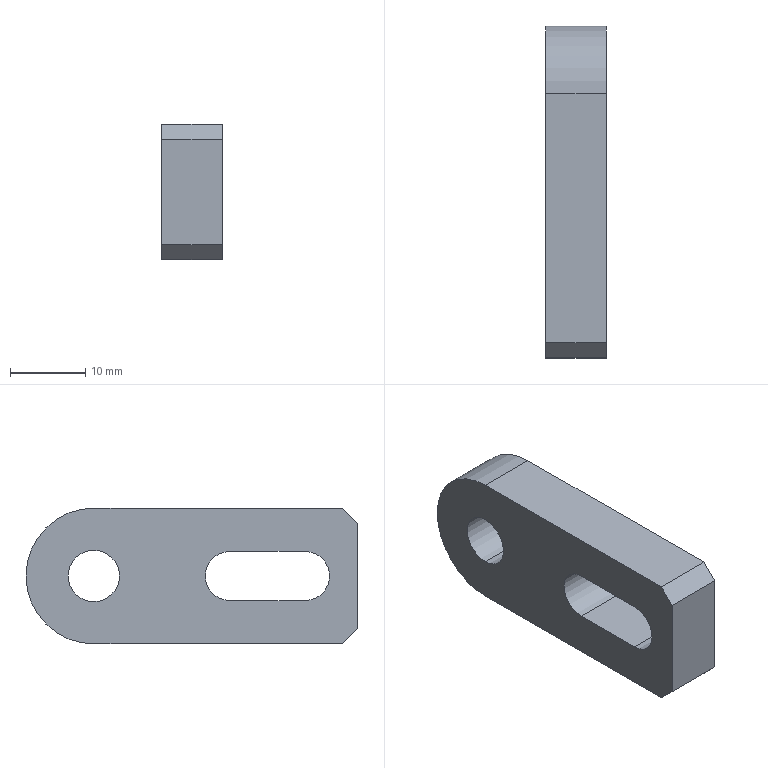Part | SolidWorks | features Chamfer 1, Extrusion 1, HoleWzd 1 | 1 solid | 14 faces | box 8 x 44 x 18 mm | volume 4950 mm3 | plane 9 | cylinder 5 | commonest cylinder face diameters 6.5 x2 6.8 x2 18 x1
STEP:
#1=CARTESIAN_POINT('',(4.,35.,3.4));
#2=VERTEX_POINT('',#1);
#3=CARTESIAN_POINT('',(4.,35.,-3.4));
#4=VERTEX_POINT('',#3);
#5=CARTESIAN_POINT('',(4.,35.,0.));
#6=DIRECTION('',(1.,0.,0.));
#7=DIRECTION('',(0.,0.,-1.));
#8=AXIS2_PLACEMENT_3D('',#5,#6,#7);
#9=CIRCLE('',#8,3.4);
#10=EDGE_CURVE('',#2,#4,#9,.T.);
#11=ORIENTED_EDGE('',*,*,#10,.T.);
#12=CARTESIAN_POINT('',(-4.,35.,-3.4));
#13=VERTEX_POINT('',#12);
#14=CARTESIAN_POINT('',(-4.,35.,-3.4));
#15=DIRECTION('',(-1.,0.,0.));
#16=VECTOR('',#15,1000.);
#17=LINE('',#14,#16);
#18=EDGE_CURVE('',#4,#13,#17,.T.);
#19=ORIENTED_EDGE('',*,*,#18,.T.);
#20=CARTESIAN_POINT('',(-4.,35.,3.4));
#21=VERTEX_POINT('',#20);
#22=CARTESIAN_POINT('',(-4.,35.,0.));
#23=DIRECTION('',(-1.,0.,0.));
#24=DIRECTION('',(0.,0.,1.));
#25=AXIS2_PLACEMENT_3D('',#22,#23,#24);
#26=CIRCLE('',#25,3.4);
#27=EDGE_CURVE('',#13,#21,#26,.T.);
#28=ORIENTED_EDGE('',*,*,#27,.T.);
#29=CARTESIAN_POINT('',(-4.,35.,3.4));
#30=DIRECTION('',(-1.,0.,0.));
#31=VECTOR('',#30,1000.);
#32=LINE('',#29,#31);
#33=EDGE_CURVE('',#2,#21,#32,.T.);
#34=ORIENTED_EDGE('',*,*,#33,.F.);
#35=EDGE_LOOP('',(#11,#19,#28,#34));
#36=FACE_OUTER_BOUND('',#35,.T.);
#37=CARTESIAN_POINT('',(-4.,35.,0.));
#38=DIRECTION('',(-1.,0.,0.));
#39=DIRECTION('',(0.,0.,1.));
#40=AXIS2_PLACEMENT_3D('',#37,#38,#39);
#41=CYLINDRICAL_SURFACE('',#40,3.4);
#42=ADVANCED_FACE('',(#36),#41,.F.);
#43=ORIENTED_EDGE('',*,*,#10,.F.);
#44=CARTESIAN_POINT('',(4.,35.,0.));
#45=DIRECTION('',(1.,0.,0.));
#46=DIRECTION('',(0.,0.,-1.));
#47=AXIS2_PLACEMENT_3D('',#44,#45,#46);
#48=CIRCLE('',#47,3.4);
#49=EDGE_CURVE('',#4,#2,#48,.T.);
#50=ORIENTED_EDGE('',*,*,#49,.F.);
#51=EDGE_LOOP('',(#43,#50));
#52=FACE_BOUND('',#51,.T.);
#53=CARTESIAN_POINT('',(4.,35.,9.));
#54=VERTEX_POINT('',#53);
#55=CARTESIAN_POINT('',(4.,2.,9.));
#56=VERTEX_POINT('',#55);
#57=CARTESIAN_POINT('',(4.,0.,9.));
#58=DIRECTION('',(0.,-1.,0.));
#59=VECTOR('',#58,1000.);
#60=LINE('',#57,#59);
#61=EDGE_CURVE('',#54,#56,#60,.T.);
#62=ORIENTED_EDGE('',*,*,#61,.T.);
#63=CARTESIAN_POINT('',(4.,0.,7.));
#64=VERTEX_POINT('',#63);
#65=CARTESIAN_POINT('',(4.,14.,21.));
#66=DIRECTION('',(0.,-0.7071,-0.7071));
#67=VECTOR('',#66,1000.);
#68=LINE('',#65,#67);
#69=EDGE_CURVE('',#56,#64,#68,.T.);
#70=ORIENTED_EDGE('',*,*,#69,.T.);
#71=CARTESIAN_POINT('',(4.,0.,-7.));
#72=VERTEX_POINT('',#71);
#73=CARTESIAN_POINT('',(4.,0.,9.));
#74=DIRECTION('',(0.,0.,-1.));
#75=VECTOR('',#74,1000.);
#76=LINE('',#73,#75);
#77=EDGE_CURVE('',#64,#72,#76,.T.);
#78=ORIENTED_EDGE('',*,*,#77,.T.);
#79=CARTESIAN_POINT('',(4.,2.,-9.));
#80=VERTEX_POINT('',#79);
#81=CARTESIAN_POINT('',(4.,14.,-21.));
#82=DIRECTION('',(0.,0.7071,-0.7071));
#83=VECTOR('',#82,1000.);
#84=LINE('',#81,#83);
#85=EDGE_CURVE('',#72,#80,#84,.T.);
#86=ORIENTED_EDGE('',*,*,#85,.T.);
#87=CARTESIAN_POINT('',(4.,35.,-9.));
#88=VERTEX_POINT('',#87);
#89=CARTESIAN_POINT('',(4.,0.,-9.));
#90=DIRECTION('',(0.,1.,0.));
#91=VECTOR('',#90,1000.);
#92=LINE('',#89,#91);
#93=EDGE_CURVE('',#80,#88,#92,.T.);
#94=ORIENTED_EDGE('',*,*,#93,.T.);
#95=CARTESIAN_POINT('',(4.,35.,0.));
#96=DIRECTION('',(1.,0.,0.));
#97=DIRECTION('',(0.,0.,-1.));
#98=AXIS2_PLACEMENT_3D('',#95,#96,#97);
#99=CIRCLE('',#98,9.);
#100=EDGE_CURVE('',#88,#54,#99,.T.);
#101=ORIENTED_EDGE('',*,*,#100,.T.);
#102=EDGE_LOOP('',(#62,#70,#78,#86,#94,#101));
#103=FACE_OUTER_BOUND('',#102,.T.);
#104=CARTESIAN_POINT('',(4.,17.,3.25));
#105=VERTEX_POINT('',#104);
#106=CARTESIAN_POINT('',(4.,7.,3.25));
#107=VERTEX_POINT('',#106);
#108=CARTESIAN_POINT('',(4.,17.,3.25));
#109=DIRECTION('',(0.,-1.,0.));
#110=VECTOR('',#109,1000.);
#111=LINE('',#108,#110);
#112=EDGE_CURVE('',#105,#107,#111,.T.);
#113=ORIENTED_EDGE('',*,*,#112,.F.);
#114=CARTESIAN_POINT('',(4.,17.,-3.25));
#115=VERTEX_POINT('',#114);
#116=CARTESIAN_POINT('',(4.,17.,0.));
#117=DIRECTION('',(1.,0.,0.));
#118=DIRECTION('',(0.,0.,-1.));
#119=AXIS2_PLACEMENT_3D('',#116,#117,#118);
#120=CIRCLE('',#119,3.25);
#121=EDGE_CURVE('',#115,#105,#120,.T.);
#122=ORIENTED_EDGE('',*,*,#121,.F.);
#123=CARTESIAN_POINT('',(4.,7.,-3.25));
#124=VERTEX_POINT('',#123);
#125=CARTESIAN_POINT('',(4.,17.,-3.25));
#126=DIRECTION('',(0.,1.,0.));
#127=VECTOR('',#126,1000.);
#128=LINE('',#125,#127);
#129=EDGE_CURVE('',#124,#115,#128,.T.);
#130=ORIENTED_EDGE('',*,*,#129,.F.);
#131=CARTESIAN_POINT('',(4.,7.,0.));
#132=DIRECTION('',(1.,0.,0.));
#133=DIRECTION('',(0.,0.,-1.));
#134=AXIS2_PLACEMENT_3D('',#131,#132,#133);
#135=CIRCLE('',#134,3.25);
#136=EDGE_CURVE('',#107,#124,#135,.T.);
#137=ORIENTED_EDGE('',*,*,#136,.F.);
#138=EDGE_LOOP('',(#113,#122,#130,#137));
#139=FACE_BOUND('',#138,.T.);
#140=CARTESIAN_POINT('',(4.,35.,0.));
#141=DIRECTION('',(1.,0.,0.));
#142=DIRECTION('',(0.,0.,-1.));
#143=AXIS2_PLACEMENT_3D('',#140,#141,#142);
#144=PLANE('',#143);
#145=ADVANCED_FACE('',(#52,#103,#139),#144,.T.);
#146=CARTESIAN_POINT('',(-4.,35.,0.));
#147=DIRECTION('',(-1.,0.,0.));
#148=DIRECTION('',(0.,0.,1.));
#149=AXIS2_PLACEMENT_3D('',#146,#147,#148);
#150=CIRCLE('',#149,3.4);
#151=EDGE_CURVE('',#21,#13,#150,.T.);
#152=ORIENTED_EDGE('',*,*,#151,.F.);
#153=ORIENTED_EDGE('',*,*,#27,.F.);
#154=EDGE_LOOP('',(#152,#153));
#155=FACE_BOUND('',#154,.T.);
#156=CARTESIAN_POINT('',(-4.,0.,7.));
#157=VERTEX_POINT('',#156);
#158=CARTESIAN_POINT('',(-4.,0.,-7.));
#159=VERTEX_POINT('',#158);
#160=CARTESIAN_POINT('',(-4.,0.,9.));
#161=DIRECTION('',(0.,0.,-1.));
#162=VECTOR('',#161,1000.);
#163=LINE('',#160,#162);
#164=EDGE_CURVE('',#157,#159,#163,.T.);
#165=ORIENTED_EDGE('',*,*,#164,.F.);
#166=CARTESIAN_POINT('',(-4.,2.,9.));
#167=VERTEX_POINT('',#166);
#168=CARTESIAN_POINT('',(-4.,0.,7.));
#169=DIRECTION('',(0.,0.7071,0.7071));
#170=VECTOR('',#169,1000.);
#171=LINE('',#168,#170);
#172=EDGE_CURVE('',#157,#167,#171,.T.);
#173=ORIENTED_EDGE('',*,*,#172,.T.);
#174=CARTESIAN_POINT('',(-4.,35.,9.));
#175=VERTEX_POINT('',#174);
#176=CARTESIAN_POINT('',(-4.,0.,9.));
#177=DIRECTION('',(0.,-1.,0.));
#178=VECTOR('',#177,1000.);
#179=LINE('',#176,#178);
#180=EDGE_CURVE('',#175,#167,#179,.T.);
#181=ORIENTED_EDGE('',*,*,#180,.F.);
#182=CARTESIAN_POINT('',(-4.,35.,-9.));
#183=VERTEX_POINT('',#182);
#184=CARTESIAN_POINT('',(-4.,35.,0.));
#185=DIRECTION('',(1.,0.,0.));
#186=DIRECTION('',(0.,0.,-1.));
#187=AXIS2_PLACEMENT_3D('',#184,#185,#186);
#188=CIRCLE('',#187,9.);
#189=EDGE_CURVE('',#183,#175,#188,.T.);
#190=ORIENTED_EDGE('',*,*,#189,.F.);
#191=CARTESIAN_POINT('',(-4.,2.,-9.));
#192=VERTEX_POINT('',#191);
#193=CARTESIAN_POINT('',(-4.,0.,-9.));
#194=DIRECTION('',(0.,1.,0.));
#195=VECTOR('',#194,1000.);
#196=LINE('',#193,#195);
#197=EDGE_CURVE('',#192,#183,#196,.T.);
#198=ORIENTED_EDGE('',*,*,#197,.F.);
#199=CARTESIAN_POINT('',(-4.,2.,-9.));
#200=DIRECTION('',(0.,-0.7071,0.7071));
#201=VECTOR('',#200,1000.);
#202=LINE('',#199,#201);
#203=EDGE_CURVE('',#192,#159,#202,.T.);
#204=ORIENTED_EDGE('',*,*,#203,.T.);
#205=EDGE_LOOP('',(#165,#173,#181,#190,#198,#204));
#206=FACE_OUTER_BOUND('',#205,.T.);
#207=CARTESIAN_POINT('',(-4.,17.,-3.25));
#208=VERTEX_POINT('',#207);
#209=CARTESIAN_POINT('',(-4.,17.,3.25));
#210=VERTEX_POINT('',#209);
#211=CARTESIAN_POINT('',(-4.,17.,0.));
#212=DIRECTION('',(1.,0.,0.));
#213=DIRECTION('',(0.,0.,-1.));
#214=AXIS2_PLACEMENT_3D('',#211,#212,#213);
#215=CIRCLE('',#214,3.25);
#216=EDGE_CURVE('',#208,#210,#215,.T.);
#217=ORIENTED_EDGE('',*,*,#216,.T.);
#218=CARTESIAN_POINT('',(-4.,7.,3.25));
#219=VERTEX_POINT('',#218);
#220=CARTESIAN_POINT('',(-4.,17.,3.25));
#221=DIRECTION('',(0.,-1.,0.));
#222=VECTOR('',#221,1000.);
#223=LINE('',#220,#222);
#224=EDGE_CURVE('',#210,#219,#223,.T.);
#225=ORIENTED_EDGE('',*,*,#224,.T.);
#226=CARTESIAN_POINT('',(-4.,7.,-3.25));
#227=VERTEX_POINT('',#226);
#228=CARTESIAN_POINT('',(-4.,7.,0.));
#229=DIRECTION('',(1.,0.,0.));
#230=DIRECTION('',(0.,0.,-1.));
#231=AXIS2_PLACEMENT_3D('',#228,#229,#230);
#232=CIRCLE('',#231,3.25);
#233=EDGE_CURVE('',#219,#227,#232,.T.);
#234=ORIENTED_EDGE('',*,*,#233,.T.);
#235=CARTESIAN_POINT('',(-4.,17.,-3.25));
#236=DIRECTION('',(0.,1.,0.));
#237=VECTOR('',#236,1000.);
#238=LINE('',#235,#237);
#239=EDGE_CURVE('',#227,#208,#238,.T.);
#240=ORIENTED_EDGE('',*,*,#239,.T.);
#241=EDGE_LOOP('',(#217,#225,#234,#240));
#242=FACE_BOUND('',#241,.T.);
#243=CARTESIAN_POINT('',(-4.,35.,0.));
#244=DIRECTION('',(1.,0.,0.));
#245=DIRECTION('',(0.,0.,-1.));
#246=AXIS2_PLACEMENT_3D('',#243,#244,#245);
#247=PLANE('',#246);
#248=ADVANCED_FACE('',(#155,#206,#242),#247,.F.);
#249=ORIENTED_EDGE('',*,*,#180,.T.);
#250=CARTESIAN_POINT('',(4.,2.,9.));
#251=DIRECTION('',(1.,0.,0.));
#252=VECTOR('',#251,1000.);
#253=LINE('',#250,#252);
#254=EDGE_CURVE('',#167,#56,#253,.T.);
#255=ORIENTED_EDGE('',*,*,#254,.T.);
#256=ORIENTED_EDGE('',*,*,#61,.F.);
#257=CARTESIAN_POINT('',(4.,35.,9.));
#258=DIRECTION('',(-1.,0.,0.));
#259=VECTOR('',#258,1000.);
#260=LINE('',#257,#259);
#261=EDGE_CURVE('',#54,#175,#260,.T.);
#262=ORIENTED_EDGE('',*,*,#261,.T.);
#263=EDGE_LOOP('',(#249,#255,#256,#262));
#264=FACE_OUTER_BOUND('',#263,.T.);
#265=CARTESIAN_POINT('',(4.,0.,9.));
#266=DIRECTION('',(0.,0.,-1.));
#267=DIRECTION('',(-1.,0.,0.));
#268=AXIS2_PLACEMENT_3D('',#265,#266,#267);
#269=PLANE('',#268);
#270=ADVANCED_FACE('',(#264),#269,.F.);
#271=ORIENTED_EDGE('',*,*,#77,.F.);
#272=CARTESIAN_POINT('',(4.,0.,7.));
#273=DIRECTION('',(-1.,0.,0.));
#274=VECTOR('',#273,1000.);
#275=LINE('',#272,#274);
#276=EDGE_CURVE('',#64,#157,#275,.T.);
#277=ORIENTED_EDGE('',*,*,#276,.T.);
#278=ORIENTED_EDGE('',*,*,#164,.T.);
#279=CARTESIAN_POINT('',(4.,0.,-7.));
#280=DIRECTION('',(1.,0.,0.));
#281=VECTOR('',#280,1000.);
#282=LINE('',#279,#281);
#283=EDGE_CURVE('',#159,#72,#282,.T.);
#284=ORIENTED_EDGE('',*,*,#283,.T.);
#285=EDGE_LOOP('',(#271,#277,#278,#284));
#286=FACE_OUTER_BOUND('',#285,.T.);
#287=CARTESIAN_POINT('',(4.,0.,9.));
#288=DIRECTION('',(0.,1.,0.));
#289=DIRECTION('',(0.,0.,1.));
#290=AXIS2_PLACEMENT_3D('',#287,#288,#289);
#291=PLANE('',#290);
#292=ADVANCED_FACE('',(#286),#291,.F.);
#293=ORIENTED_EDGE('',*,*,#93,.F.);
#294=CARTESIAN_POINT('',(4.,2.,-9.));
#295=DIRECTION('',(-1.,0.,0.));
#296=VECTOR('',#295,1000.);
#297=LINE('',#294,#296);
#298=EDGE_CURVE('',#80,#192,#297,.T.);
#299=ORIENTED_EDGE('',*,*,#298,.T.);
#300=ORIENTED_EDGE('',*,*,#197,.T.);
#301=CARTESIAN_POINT('',(4.,35.,-9.));
#302=DIRECTION('',(-1.,0.,0.));
#303=VECTOR('',#302,1000.);
#304=LINE('',#301,#303);
#305=EDGE_CURVE('',#88,#183,#304,.T.);
#306=ORIENTED_EDGE('',*,*,#305,.F.);
#307=EDGE_LOOP('',(#293,#299,#300,#306));
#308=FACE_OUTER_BOUND('',#307,.T.);
#309=CARTESIAN_POINT('',(4.,0.,-9.));
#310=DIRECTION('',(0.,0.,1.));
#311=DIRECTION('',(1.,0.,0.));
#312=AXIS2_PLACEMENT_3D('',#309,#310,#311);
#313=PLANE('',#312);
#314=ADVANCED_FACE('',(#308),#313,.F.);
#315=ORIENTED_EDGE('',*,*,#189,.T.);
#316=ORIENTED_EDGE('',*,*,#261,.F.);
#317=ORIENTED_EDGE('',*,*,#100,.F.);
#318=ORIENTED_EDGE('',*,*,#305,.T.);
#319=EDGE_LOOP('',(#315,#316,#317,#318));
#320=FACE_OUTER_BOUND('',#319,.T.);
#321=CARTESIAN_POINT('',(4.,35.,0.));
#322=DIRECTION('',(-1.,0.,0.));
#323=DIRECTION('',(0.,0.,1.));
#324=AXIS2_PLACEMENT_3D('',#321,#322,#323);
#325=CYLINDRICAL_SURFACE('',#324,9.);
#326=ADVANCED_FACE('',(#320),#325,.T.);
#327=ORIENTED_EDGE('',*,*,#216,.F.);
#328=CARTESIAN_POINT('',(4.,17.,-3.25));
#329=DIRECTION('',(-1.,0.,0.));
#330=VECTOR('',#329,1000.);
#331=LINE('',#328,#330);
#332=EDGE_CURVE('',#115,#208,#331,.T.);
#333=ORIENTED_EDGE('',*,*,#332,.F.);
#334=ORIENTED_EDGE('',*,*,#121,.T.);
#335=CARTESIAN_POINT('',(4.,17.,3.25));
#336=DIRECTION('',(-1.,0.,0.));
#337=VECTOR('',#336,1000.);
#338=LINE('',#335,#337);
#339=EDGE_CURVE('',#105,#210,#338,.T.);
#340=ORIENTED_EDGE('',*,*,#339,.T.);
#341=EDGE_LOOP('',(#327,#333,#334,#340));
#342=FACE_OUTER_BOUND('',#341,.T.);
#343=CARTESIAN_POINT('',(4.,17.,0.));
#344=DIRECTION('',(-1.,0.,0.));
#345=DIRECTION('',(0.,0.,1.));
#346=AXIS2_PLACEMENT_3D('',#343,#344,#345);
#347=CYLINDRICAL_SURFACE('',#346,3.25);
#348=ADVANCED_FACE('',(#342),#347,.F.);
#349=ORIENTED_EDGE('',*,*,#224,.F.);
#350=ORIENTED_EDGE('',*,*,#339,.F.);
#351=ORIENTED_EDGE('',*,*,#112,.T.);
#352=CARTESIAN_POINT('',(4.,7.,3.25));
#353=DIRECTION('',(-1.,0.,0.));
#354=VECTOR('',#353,1000.);
#355=LINE('',#352,#354);
#356=EDGE_CURVE('',#107,#219,#355,.T.);
#357=ORIENTED_EDGE('',*,*,#356,.T.);
#358=EDGE_LOOP('',(#349,#350,#351,#357));
#359=FACE_OUTER_BOUND('',#358,.T.);
#360=CARTESIAN_POINT('',(4.,17.,3.25));
#361=DIRECTION('',(0.,0.,-1.));
#362=DIRECTION('',(0.,1.,0.));
#363=AXIS2_PLACEMENT_3D('',#360,#361,#362);
#364=PLANE('',#363);
#365=ADVANCED_FACE('',(#359),#364,.T.);
#366=ORIENTED_EDGE('',*,*,#233,.F.);
#367=ORIENTED_EDGE('',*,*,#356,.F.);
#368=ORIENTED_EDGE('',*,*,#136,.T.);
#369=CARTESIAN_POINT('',(4.,7.,-3.25));
#370=DIRECTION('',(-1.,0.,0.));
#371=VECTOR('',#370,1000.);
#372=LINE('',#369,#371);
#373=EDGE_CURVE('',#124,#227,#372,.T.);
#374=ORIENTED_EDGE('',*,*,#373,.T.);
#375=EDGE_LOOP('',(#366,#367,#368,#374));
#376=FACE_OUTER_BOUND('',#375,.T.);
#377=CARTESIAN_POINT('',(4.,7.,0.));
#378=DIRECTION('',(-1.,0.,0.));
#379=DIRECTION('',(0.,0.,1.));
#380=AXIS2_PLACEMENT_3D('',#377,#378,#379);
#381=CYLINDRICAL_SURFACE('',#380,3.25);
#382=ADVANCED_FACE('',(#376),#381,.F.);
#383=ORIENTED_EDGE('',*,*,#239,.F.);
#384=ORIENTED_EDGE('',*,*,#373,.F.);
#385=ORIENTED_EDGE('',*,*,#129,.T.);
#386=ORIENTED_EDGE('',*,*,#332,.T.);
#387=EDGE_LOOP('',(#383,#384,#385,#386));
#388=FACE_OUTER_BOUND('',#387,.T.);
#389=CARTESIAN_POINT('',(4.,17.,-3.25));
#390=DIRECTION('',(0.,0.,1.));
#391=DIRECTION('',(0.,-1.,0.));
#392=AXIS2_PLACEMENT_3D('',#389,#390,#391);
#393=PLANE('',#392);
#394=ADVANCED_FACE('',(#388),#393,.T.);
#395=ORIENTED_EDGE('',*,*,#18,.F.);
#396=ORIENTED_EDGE('',*,*,#49,.T.);
#397=ORIENTED_EDGE('',*,*,#33,.T.);
#398=ORIENTED_EDGE('',*,*,#151,.T.);
#399=EDGE_LOOP('',(#395,#396,#397,#398));
#400=FACE_OUTER_BOUND('',#399,.T.);
#401=CARTESIAN_POINT('',(-4.,35.,0.));
#402=DIRECTION('',(-1.,0.,0.));
#403=DIRECTION('',(0.,0.,1.));
#404=AXIS2_PLACEMENT_3D('',#401,#402,#403);
#405=CYLINDRICAL_SURFACE('',#404,3.4);
#406=ADVANCED_FACE('',(#400),#405,.F.);
#407=ORIENTED_EDGE('',*,*,#69,.F.);
#408=ORIENTED_EDGE('',*,*,#254,.F.);
#409=ORIENTED_EDGE('',*,*,#172,.F.);
#410=ORIENTED_EDGE('',*,*,#276,.F.);
#411=EDGE_LOOP('',(#407,#408,#409,#410));
#412=FACE_OUTER_BOUND('',#411,.T.);
#413=CARTESIAN_POINT('',(4.,0.,7.));
#414=DIRECTION('',(0.,0.7071,-0.7071));
#415=DIRECTION('',(-1.,0.,0.));
#416=AXIS2_PLACEMENT_3D('',#413,#414,#415);
#417=PLANE('',#416);
#418=ADVANCED_FACE('',(#412),#417,.F.);
#419=ORIENTED_EDGE('',*,*,#85,.F.);
#420=ORIENTED_EDGE('',*,*,#283,.F.);
#421=ORIENTED_EDGE('',*,*,#203,.F.);
#422=ORIENTED_EDGE('',*,*,#298,.F.);
#423=EDGE_LOOP('',(#419,#420,#421,#422));
#424=FACE_OUTER_BOUND('',#423,.T.);
#425=CARTESIAN_POINT('',(4.,2.,-9.));
#426=DIRECTION('',(0.,0.7071,0.7071));
#427=DIRECTION('',(-1.,0.,0.));
#428=AXIS2_PLACEMENT_3D('',#425,#426,#427);
#429=PLANE('',#428);
#430=ADVANCED_FACE('',(#424),#429,.F.);
#431=CLOSED_SHELL('',(#42,#145,#248,#270,#292,#314,#326,#348,#365,#382,#394,#406,#418,#430));
#432=MANIFOLD_SOLID_BREP('',#431);
#433=CARTESIAN_POINT('',(0.,0.,0.));
#434=DIRECTION('',(0.,0.,1.));
#435=DIRECTION('',(1.,0.,0.));
#436=AXIS2_PLACEMENT_3D('',#433,#434,#435);
#437=(LENGTH_UNIT()NAMED_UNIT(*)SI_UNIT(.MILLI.,.METRE.));
#438=UNCERTAINTY_MEASURE_WITH_UNIT(LENGTH_MEASURE(0.00001),#437,'','');
#439=(NAMED_UNIT(*)PLANE_ANGLE_UNIT()SI_UNIT($,.RADIAN.));
#440=(NAMED_UNIT(*)SI_UNIT($,.STERADIAN.)SOLID_ANGLE_UNIT());
#441=(GEOMETRIC_REPRESENTATION_CONTEXT(3)GLOBAL_UNCERTAINTY_ASSIGNED_CONTEXT((#438))GLOBAL_UNIT_ASSIGNED_CONTEXT((#437,#439,#440))REPRESENTATION_CONTEXT('',''));
#442=ADVANCED_BREP_SHAPE_REPRESENTATION('',(#432,#436),#441);